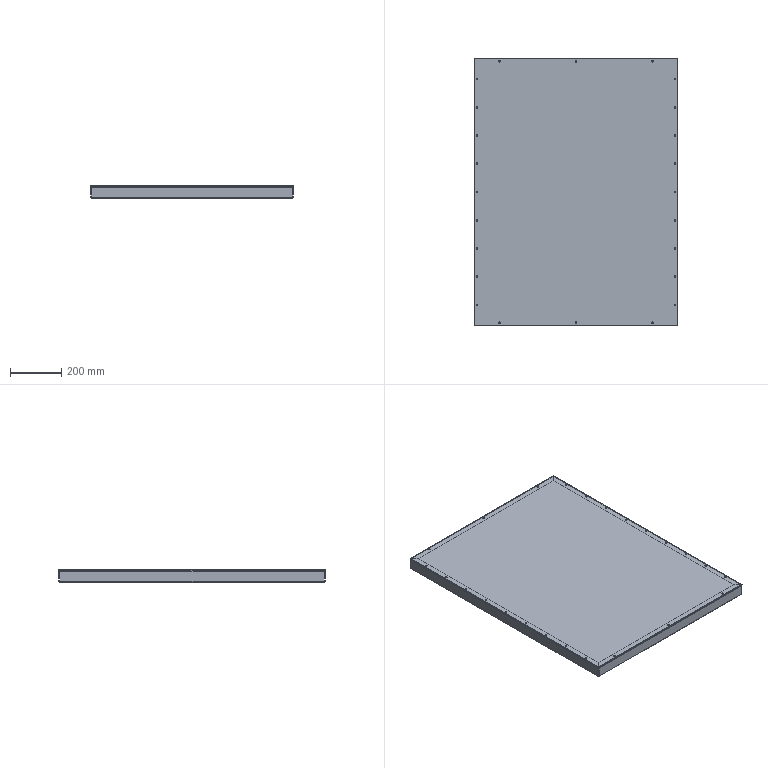Part | SolidWorks | 2 solids | 172 faces | box 794 x 1043 x 47 mm | volume 4274247 mm3 | cylinder 112 | plane 44 | spline 16 | commonest cylinder face diameters 5 x48 6.5 x48 1.473 x8 6.473 x8